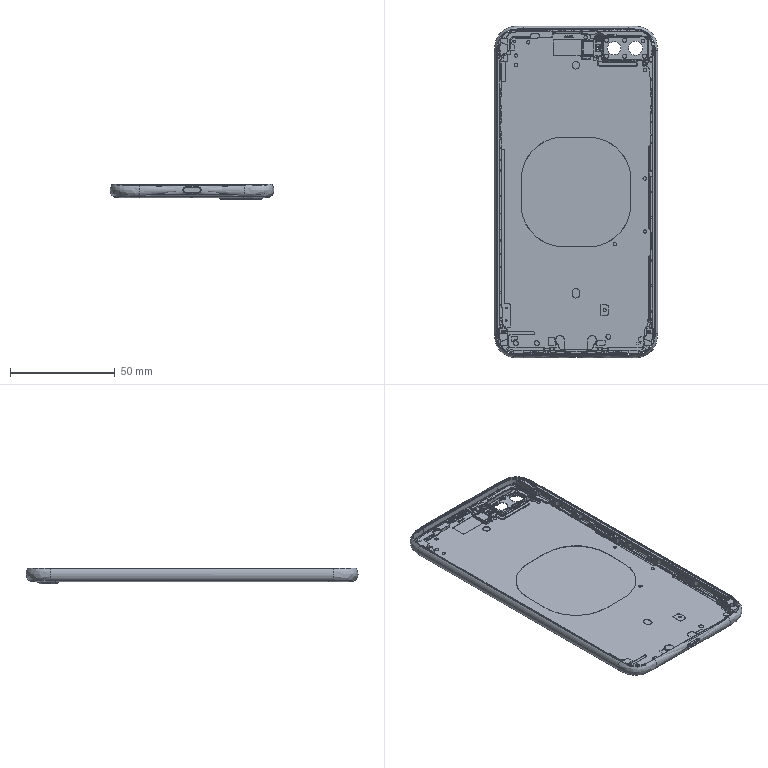Part | SolidWorks | features BaseBody 488, RefSurface 10, DeleteBody 7 | 58 solids | 4635 faces | volume 15410 mm3 | plane 1737 | cylinder 1524 | spline 971 | cone 403 | commonest cylinder face diameters 0.2 x149 1.1 x120 1 x114 2.2 x87 1.5 x83 0.08 x82